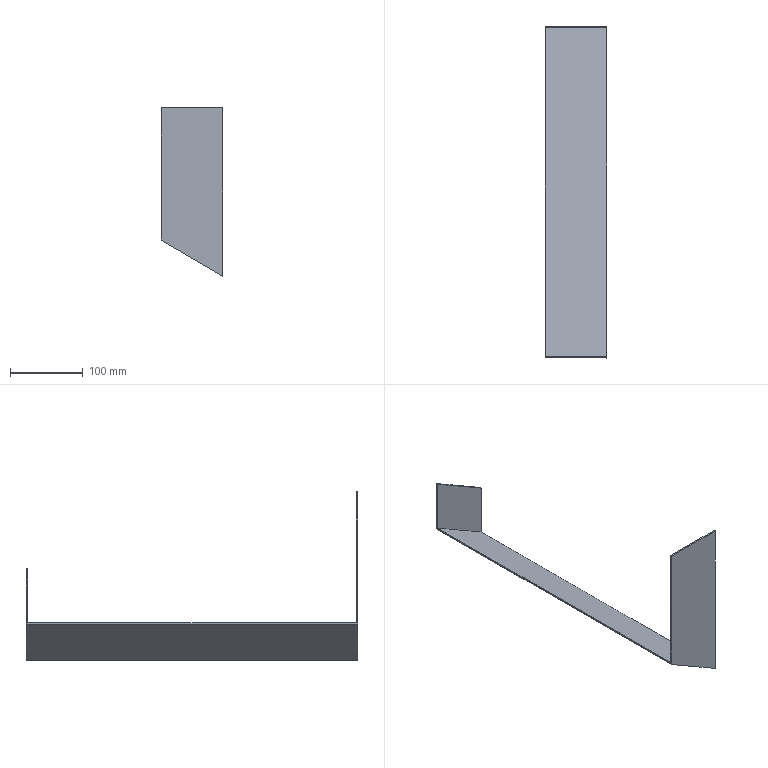Part | STEP file | lll_id4134_x_t | 1 solid | 11 faces | box 85 x 455 x 230.884 mm | volume 136566 mm3 | plane 11
STEP:
#1=CARTESIAN_POINT('',(4052.435,18.,-0.5));
#2=VERTEX_POINT('',#1);
#3=CARTESIAN_POINT('',(4052.435,16.,-0.5));
#4=VERTEX_POINT('',#3);
#5=CARTESIAN_POINT('',(4052.435,0.,-0.5));
#6=DIRECTION('',(0.,-1.,0.));
#7=VECTOR('',#6,1.);
#8=LINE('',#5,#7);
#9=EDGE_CURVE('',#2,#4,#8,.T.);
#10=ORIENTED_EDGE('',*,*,#9,.T.);
#11=CARTESIAN_POINT('',(4052.435,16.,-231.384));
#12=VERTEX_POINT('',#11);
#13=CARTESIAN_POINT('',(4052.435,16.,-250.));
#14=DIRECTION('',(0.,0.,-1.));
#15=VECTOR('',#14,1.);
#16=LINE('',#13,#15);
#17=EDGE_CURVE('',#4,#12,#16,.T.);
#18=ORIENTED_EDGE('',*,*,#17,.T.);
#19=CARTESIAN_POINT('',(4052.435,471.,-231.384));
#20=VERTEX_POINT('',#19);
#21=CARTESIAN_POINT('',(4052.435,0.,-231.384));
#22=DIRECTION('',(0.,-1.,0.));
#23=VECTOR('',#22,1.);
#24=LINE('',#21,#23);
#25=EDGE_CURVE('',#20,#12,#24,.T.);
#26=ORIENTED_EDGE('',*,*,#25,.F.);
#27=CARTESIAN_POINT('',(4052.435,471.,-155.174));
#28=VERTEX_POINT('',#27);
#29=CARTESIAN_POINT('',(4052.435,471.,-180.));
#30=DIRECTION('',(0.,0.,-1.));
#31=VECTOR('',#30,1.);
#32=LINE('',#29,#31);
#33=EDGE_CURVE('',#28,#20,#32,.T.);
#34=ORIENTED_EDGE('',*,*,#33,.F.);
#35=CARTESIAN_POINT('',(4052.435,469.,-155.174));
#36=VERTEX_POINT('',#35);
#37=CARTESIAN_POINT('',(4052.435,471.,-155.174));
#38=DIRECTION('',(0.,1.,0.));
#39=VECTOR('',#38,1.);
#40=LINE('',#37,#39);
#41=EDGE_CURVE('',#36,#28,#40,.T.);
#42=ORIENTED_EDGE('',*,*,#41,.F.);
#43=CARTESIAN_POINT('',(4052.435,469.,-229.075));
#44=VERTEX_POINT('',#43);
#45=CARTESIAN_POINT('',(4052.435,469.,-250.));
#46=DIRECTION('',(0.,0.,1.));
#47=VECTOR('',#46,1.);
#48=LINE('',#45,#47);
#49=EDGE_CURVE('',#44,#36,#48,.T.);
#50=ORIENTED_EDGE('',*,*,#49,.F.);
#51=CARTESIAN_POINT('',(4052.435,18.,-229.075));
#52=VERTEX_POINT('',#51);
#53=CARTESIAN_POINT('',(4052.435,0.,-229.075));
#54=DIRECTION('',(0.,-1.,0.));
#55=VECTOR('',#54,1.);
#56=LINE('',#53,#55);
#57=EDGE_CURVE('',#44,#52,#56,.T.);
#58=ORIENTED_EDGE('',*,*,#57,.T.);
#59=CARTESIAN_POINT('',(4052.435,18.,-0.5));
#60=DIRECTION('',(0.,0.,1.));
#61=VECTOR('',#60,1.);
#62=LINE('',#59,#61);
#63=EDGE_CURVE('',#52,#2,#62,.T.);
#64=ORIENTED_EDGE('',*,*,#63,.T.);
#65=EDGE_LOOP('',(#10,#18,#26,#34,#42,#50,#58,#64));
#66=FACE_OUTER_BOUND('',#65,.T.);
#67=CARTESIAN_POINT('',(4052.435,0.,-250.));
#68=DIRECTION('',(1.,0.,0.));
#69=DIRECTION('',(0.,0.,-1.));
#70=AXIS2_PLACEMENT_3D('',#67,#68,#69);
#71=PLANE('',#70);
#72=ADVANCED_FACE('',(#66),#71,.T.);
#73=CARTESIAN_POINT('',(3967.435,16.,-0.5));
#74=VERTEX_POINT('',#73);
#75=CARTESIAN_POINT('',(3967.435,16.,-180.));
#76=VERTEX_POINT('',#75);
#77=CARTESIAN_POINT('',(3967.435,16.,-0.5));
#78=DIRECTION('',(0.,0.,-1.));
#79=VECTOR('',#78,1.);
#80=LINE('',#77,#79);
#81=EDGE_CURVE('',#74,#76,#80,.T.);
#82=ORIENTED_EDGE('',*,*,#81,.F.);
#83=CARTESIAN_POINT('',(3967.435,18.,-0.5));
#84=VERTEX_POINT('',#83);
#85=CARTESIAN_POINT('',(3967.435,5.,-0.5));
#86=DIRECTION('',(0.,1.,0.));
#87=VECTOR('',#86,1.);
#88=LINE('',#85,#87);
#89=EDGE_CURVE('',#74,#84,#88,.T.);
#90=ORIENTED_EDGE('',*,*,#89,.T.);
#91=CARTESIAN_POINT('',(3967.435,18.,-180.));
#92=VERTEX_POINT('',#91);
#93=CARTESIAN_POINT('',(3967.435,18.,-0.5));
#94=DIRECTION('',(0.,0.,-1.));
#95=VECTOR('',#94,1.);
#96=LINE('',#93,#95);
#97=EDGE_CURVE('',#84,#92,#96,.T.);
#98=ORIENTED_EDGE('',*,*,#97,.T.);
#99=CARTESIAN_POINT('',(3967.435,-600.,-180.));
#100=DIRECTION('',(0.,1.,0.));
#101=VECTOR('',#100,1.);
#102=LINE('',#99,#101);
#103=EDGE_CURVE('',#76,#92,#102,.T.);
#104=ORIENTED_EDGE('',*,*,#103,.F.);
#105=EDGE_LOOP('',(#82,#90,#98,#104));
#106=FACE_OUTER_BOUND('',#105,.T.);
#107=CARTESIAN_POINT('',(3967.435,5.,-160.));
#108=DIRECTION('',(1.,0.,0.));
#109=DIRECTION('',(0.,0.,-1.));
#110=AXIS2_PLACEMENT_3D('',#107,#108,#109);
#111=PLANE('',#110);
#112=ADVANCED_FACE('',(#106),#111,.F.);
#113=ORIENTED_EDGE('',*,*,#103,.T.);
#114=CARTESIAN_POINT('',(3967.435,469.,-180.));
#115=VERTEX_POINT('',#114);
#116=CARTESIAN_POINT('',(3967.435,-600.,-180.));
#117=DIRECTION('',(0.,1.,0.));
#118=VECTOR('',#117,1.);
#119=LINE('',#116,#118);
#120=EDGE_CURVE('',#92,#115,#119,.T.);
#121=ORIENTED_EDGE('',*,*,#120,.T.);
#122=CARTESIAN_POINT('',(3967.435,469.,-106.099));
#123=VERTEX_POINT('',#122);
#124=CARTESIAN_POINT('',(3967.435,469.,-180.));
#125=DIRECTION('',(0.,0.,-1.));
#126=VECTOR('',#125,1.);
#127=LINE('',#124,#126);
#128=EDGE_CURVE('',#123,#115,#127,.T.);
#129=ORIENTED_EDGE('',*,*,#128,.F.);
#130=CARTESIAN_POINT('',(3967.435,471.,-106.099));
#131=VERTEX_POINT('',#130);
#132=CARTESIAN_POINT('',(3967.435,0.,-106.099));
#133=DIRECTION('',(0.,-1.,0.));
#134=VECTOR('',#133,1.);
#135=LINE('',#132,#134);
#136=EDGE_CURVE('',#131,#123,#135,.T.);
#137=ORIENTED_EDGE('',*,*,#136,.F.);
#138=CARTESIAN_POINT('',(3967.435,471.,-182.309));
#139=VERTEX_POINT('',#138);
#140=CARTESIAN_POINT('',(3967.435,471.,-180.));
#141=DIRECTION('',(0.,0.,-1.));
#142=VECTOR('',#141,1.);
#143=LINE('',#140,#142);
#144=EDGE_CURVE('',#131,#139,#143,.T.);
#145=ORIENTED_EDGE('',*,*,#144,.T.);
#146=CARTESIAN_POINT('',(3967.435,16.,-182.309));
#147=VERTEX_POINT('',#146);
#148=CARTESIAN_POINT('',(3967.435,-600.,-182.309));
#149=DIRECTION('',(0.,1.,0.));
#150=VECTOR('',#149,1.);
#151=LINE('',#148,#150);
#152=EDGE_CURVE('',#147,#139,#151,.T.);
#153=ORIENTED_EDGE('',*,*,#152,.F.);
#154=CARTESIAN_POINT('',(3967.435,16.,-131.405));
#155=DIRECTION('',(0.,0.,1.));
#156=VECTOR('',#155,1.);
#157=LINE('',#154,#156);
#158=EDGE_CURVE('',#147,#76,#157,.T.);
#159=ORIENTED_EDGE('',*,*,#158,.T.);
#160=EDGE_LOOP('',(#113,#121,#129,#137,#145,#153,#159));
#161=FACE_OUTER_BOUND('',#160,.T.);
#162=CARTESIAN_POINT('',(3967.435,0.,-160.));
#163=DIRECTION('',(1.,0.,0.));
#164=DIRECTION('',(0.,0.,-1.));
#165=AXIS2_PLACEMENT_3D('',#162,#163,#164);
#166=PLANE('',#165);
#167=ADVANCED_FACE('',(#161),#166,.F.);
#168=ORIENTED_EDGE('',*,*,#25,.T.);
#169=CARTESIAN_POINT('',(3966.435,16.,-181.732));
#170=DIRECTION('',(-0.866,0.,0.5));
#171=VECTOR('',#170,1.);
#172=LINE('',#169,#171);
#173=EDGE_CURVE('',#12,#147,#172,.T.);
#174=ORIENTED_EDGE('',*,*,#173,.T.);
#175=ORIENTED_EDGE('',*,*,#152,.T.);
#176=CARTESIAN_POINT('',(3966.435,471.,-181.732));
#177=DIRECTION('',(0.866,0.,-0.5));
#178=VECTOR('',#177,1.);
#179=LINE('',#176,#178);
#180=EDGE_CURVE('',#139,#20,#179,.T.);
#181=ORIENTED_EDGE('',*,*,#180,.T.);
#182=EDGE_LOOP('',(#168,#174,#175,#181));
#183=FACE_OUTER_BOUND('',#182,.T.);
#184=CARTESIAN_POINT('',(3966.435,-600.,-181.732));
#185=DIRECTION('',(0.5,0.,0.866));
#186=DIRECTION('',(0.866,0.,-0.5));
#187=AXIS2_PLACEMENT_3D('',#184,#185,#186);
#188=PLANE('',#187);
#189=ADVANCED_FACE('',(#183),#188,.F.);
#190=ORIENTED_EDGE('',*,*,#180,.F.);
#191=ORIENTED_EDGE('',*,*,#144,.F.);
#192=CARTESIAN_POINT('',(3999.435,471.,-124.574));
#193=DIRECTION('',(0.866,0.,-0.5));
#194=VECTOR('',#193,1.);
#195=LINE('',#192,#194);
#196=EDGE_CURVE('',#131,#28,#195,.T.);
#197=ORIENTED_EDGE('',*,*,#196,.T.);
#198=ORIENTED_EDGE('',*,*,#33,.T.);
#199=EDGE_LOOP('',(#190,#191,#197,#198));
#200=FACE_OUTER_BOUND('',#199,.T.);
#201=CARTESIAN_POINT('',(3967.435,471.,-180.));
#202=DIRECTION('',(0.,-1.,0.));
#203=DIRECTION('',(-0.866,0.,0.5));
#204=AXIS2_PLACEMENT_3D('',#201,#202,#203);
#205=PLANE('',#204);
#206=ADVANCED_FACE('',(#200),#205,.F.);
#207=ORIENTED_EDGE('',*,*,#196,.F.);
#208=ORIENTED_EDGE('',*,*,#136,.T.);
#209=CARTESIAN_POINT('',(3999.435,469.,-124.574));
#210=DIRECTION('',(0.866,0.,-0.5));
#211=VECTOR('',#210,1.);
#212=LINE('',#209,#211);
#213=EDGE_CURVE('',#123,#36,#212,.T.);
#214=ORIENTED_EDGE('',*,*,#213,.T.);
#215=ORIENTED_EDGE('',*,*,#41,.T.);
#216=EDGE_LOOP('',(#207,#208,#214,#215));
#217=FACE_OUTER_BOUND('',#216,.T.);
#218=CARTESIAN_POINT('',(3999.435,471.,-124.574));
#219=DIRECTION('',(-0.5,0.,-0.866));
#220=DIRECTION('',(-0.866,0.,0.5));
#221=AXIS2_PLACEMENT_3D('',#218,#219,#220);
#222=PLANE('',#221);
#223=ADVANCED_FACE('',(#217),#222,.F.);
#224=CARTESIAN_POINT('',(3967.435,469.,-180.));
#225=DIRECTION('',(0.866,0.,-0.5));
#226=VECTOR('',#225,1.);
#227=LINE('',#224,#226);
#228=EDGE_CURVE('',#115,#44,#227,.T.);
#229=ORIENTED_EDGE('',*,*,#228,.F.);
#230=ORIENTED_EDGE('',*,*,#120,.F.);
#231=CARTESIAN_POINT('',(3967.435,18.,-180.));
#232=DIRECTION('',(-0.866,0.,0.5));
#233=VECTOR('',#232,1.);
#234=LINE('',#231,#233);
#235=EDGE_CURVE('',#52,#92,#234,.T.);
#236=ORIENTED_EDGE('',*,*,#235,.F.);
#237=ORIENTED_EDGE('',*,*,#57,.F.);
#238=EDGE_LOOP('',(#229,#230,#236,#237));
#239=FACE_OUTER_BOUND('',#238,.T.);
#240=CARTESIAN_POINT('',(3967.435,-600.,-180.));
#241=DIRECTION('',(0.5,0.,0.866));
#242=DIRECTION('',(0.866,0.,-0.5));
#243=AXIS2_PLACEMENT_3D('',#240,#241,#242);
#244=PLANE('',#243);
#245=ADVANCED_FACE('',(#239),#244,.T.);
#246=ORIENTED_EDGE('',*,*,#63,.F.);
#247=ORIENTED_EDGE('',*,*,#235,.T.);
#248=ORIENTED_EDGE('',*,*,#97,.F.);
#249=CARTESIAN_POINT('',(4031.,18.,-0.5));
#250=DIRECTION('',(-1.,0.,0.));
#251=VECTOR('',#250,1.);
#252=LINE('',#249,#251);
#253=EDGE_CURVE('',#2,#84,#252,.T.);
#254=ORIENTED_EDGE('',*,*,#253,.F.);
#255=EDGE_LOOP('',(#246,#247,#248,#254));
#256=FACE_OUTER_BOUND('',#255,.T.);
#257=CARTESIAN_POINT('',(4031.,18.,-0.5));
#258=DIRECTION('',(0.,-1.,0.));
#259=DIRECTION('',(0.,0.,-1.));
#260=AXIS2_PLACEMENT_3D('',#257,#258,#259);
#261=PLANE('',#260);
#262=ADVANCED_FACE('',(#256),#261,.F.);
#263=ORIENTED_EDGE('',*,*,#253,.T.);
#264=ORIENTED_EDGE('',*,*,#89,.F.);
#265=CARTESIAN_POINT('',(4031.,16.,-0.5));
#266=DIRECTION('',(-1.,0.,0.));
#267=VECTOR('',#266,1.);
#268=LINE('',#265,#267);
#269=EDGE_CURVE('',#4,#74,#268,.T.);
#270=ORIENTED_EDGE('',*,*,#269,.F.);
#271=ORIENTED_EDGE('',*,*,#9,.F.);
#272=EDGE_LOOP('',(#263,#264,#270,#271));
#273=FACE_OUTER_BOUND('',#272,.T.);
#274=CARTESIAN_POINT('',(4031.,16.,-0.5));
#275=DIRECTION('',(0.,0.,1.));
#276=DIRECTION('',(-1.,0.,0.));
#277=AXIS2_PLACEMENT_3D('',#274,#275,#276);
#278=PLANE('',#277);
#279=ADVANCED_FACE('',(#273),#278,.T.);
#280=ORIENTED_EDGE('',*,*,#49,.T.);
#281=ORIENTED_EDGE('',*,*,#213,.F.);
#282=ORIENTED_EDGE('',*,*,#128,.T.);
#283=ORIENTED_EDGE('',*,*,#228,.T.);
#284=EDGE_LOOP('',(#280,#281,#282,#283));
#285=FACE_OUTER_BOUND('',#284,.T.);
#286=CARTESIAN_POINT('',(3967.435,469.,-180.));
#287=DIRECTION('',(0.,-1.,0.));
#288=DIRECTION('',(-0.866,0.,0.5));
#289=AXIS2_PLACEMENT_3D('',#286,#287,#288);
#290=PLANE('',#289);
#291=ADVANCED_FACE('',(#285),#290,.T.);
#292=ORIENTED_EDGE('',*,*,#269,.T.);
#293=ORIENTED_EDGE('',*,*,#81,.T.);
#294=ORIENTED_EDGE('',*,*,#158,.F.);
#295=ORIENTED_EDGE('',*,*,#173,.F.);
#296=ORIENTED_EDGE('',*,*,#17,.F.);
#297=EDGE_LOOP('',(#292,#293,#294,#295,#296));
#298=FACE_OUTER_BOUND('',#297,.T.);
#299=CARTESIAN_POINT('',(4036.718,16.,-131.405));
#300=DIRECTION('',(0.,-1.,0.));
#301=DIRECTION('',(0.,0.,1.));
#302=AXIS2_PLACEMENT_3D('',#299,#300,#301);
#303=PLANE('',#302);
#304=ADVANCED_FACE('',(#298),#303,.T.);
#305=CLOSED_SHELL('',(#72,#112,#167,#189,#206,#223,#245,#262,#279,#291,#304));
#306=MANIFOLD_SOLID_BREP('',#305);
#307=(LENGTH_UNIT()NAMED_UNIT(*)SI_UNIT(.MILLI.,.METRE.));
#308=UNCERTAINTY_MEASURE_WITH_UNIT(LENGTH_MEASURE(0.00002),#307,'','');
#309=(NAMED_UNIT(*)PLANE_ANGLE_UNIT()SI_UNIT($,.RADIAN.));
#310=PLANE_ANGLE_MEASURE_WITH_UNIT(PLANE_ANGLE_MEASURE(0.01745),#309);
#311=DIMENSIONAL_EXPONENTS(0.,0.,0.,0.,0.,0.,0.);
#312=(CONVERSION_BASED_UNIT('DEGREE',#310)NAMED_UNIT(#311)PLANE_ANGLE_UNIT());
#313=(NAMED_UNIT(*)SI_UNIT($,.STERADIAN.)SOLID_ANGLE_UNIT());
#314=(GEOMETRIC_REPRESENTATION_CONTEXT(3)GLOBAL_UNCERTAINTY_ASSIGNED_CONTEXT((#308))GLOBAL_UNIT_ASSIGNED_CONTEXT((#307,#312,#313))REPRESENTATION_CONTEXT('',''));
#315=ADVANCED_BREP_SHAPE_REPRESENTATION('',(#306),#314);